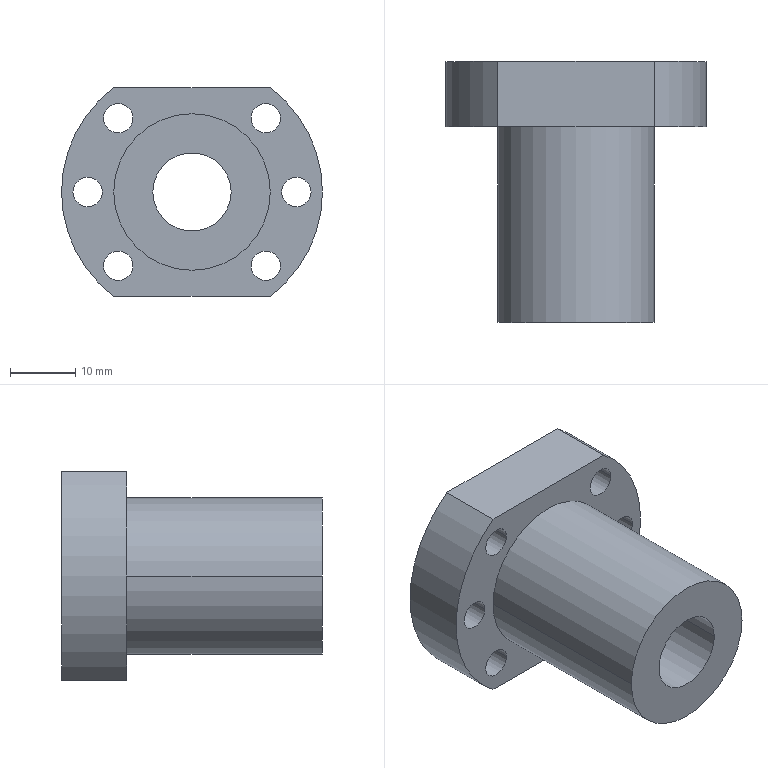Part | SolidWorks | features BaseBody 1 | 1 solid | 24 faces | box 40 x 40 x 32 mm | volume 19352 mm3 | cylinder 19 | plane 5 | commonest cylinder face diameters 4.5 x12 40 x3 12 x2 24 x2
STEP:
#1=CARTESIAN_POINT('',(-12.,-35.,0.));
#2=VERTEX_POINT('',#1);
#3=CARTESIAN_POINT('',(12.,-35.,0.));
#4=VERTEX_POINT('',#3);
#5=CARTESIAN_POINT('',(0.,-35.,0.));
#6=DIRECTION('',(0.,1.,0.));
#7=DIRECTION('',(-1.,0.,0.));
#8=AXIS2_PLACEMENT_3D('',#5,#6,#7);
#9=CIRCLE('',#8,12.);
#10=EDGE_CURVE('',#2,#4,#9,.T.);
#11=ORIENTED_EDGE('',*,*,#10,.T.);
#12=CARTESIAN_POINT('',(12.,-5.,0.));
#13=VERTEX_POINT('',#12);
#14=CARTESIAN_POINT('',(12.,-35.,0.));
#15=DIRECTION('',(0.,1.,0.));
#16=VECTOR('',#15,1000.);
#17=LINE('',#14,#16);
#18=EDGE_CURVE('',#4,#13,#17,.T.);
#19=ORIENTED_EDGE('',*,*,#18,.T.);
#20=CARTESIAN_POINT('',(-12.,-5.,0.));
#21=VERTEX_POINT('',#20);
#22=CARTESIAN_POINT('',(0.,-5.,0.));
#23=DIRECTION('',(0.,-1.,0.));
#24=DIRECTION('',(-1.,0.,0.));
#25=AXIS2_PLACEMENT_3D('',#22,#23,#24);
#26=CIRCLE('',#25,12.);
#27=EDGE_CURVE('',#13,#21,#26,.T.);
#28=ORIENTED_EDGE('',*,*,#27,.T.);
#29=CARTESIAN_POINT('',(-12.,-35.,0.));
#30=DIRECTION('',(0.,1.,0.));
#31=VECTOR('',#30,1000.);
#32=LINE('',#29,#31);
#33=EDGE_CURVE('',#2,#21,#32,.T.);
#34=ORIENTED_EDGE('',*,*,#33,.F.);
#35=EDGE_LOOP('',(#11,#19,#28,#34));
#36=FACE_OUTER_BOUND('',#35,.T.);
#37=CARTESIAN_POINT('',(0.,-35.,0.));
#38=DIRECTION('',(0.,1.,0.));
#39=DIRECTION('',(-1.,0.,0.));
#40=AXIS2_PLACEMENT_3D('',#37,#38,#39);
#41=CYLINDRICAL_SURFACE('',#40,12.);
#42=ADVANCED_FACE('',(#36),#41,.T.);
#43=CARTESIAN_POINT('',(12.,5.,-16.));
#44=VERTEX_POINT('',#43);
#45=CARTESIAN_POINT('',(20.,5.,0.));
#46=VERTEX_POINT('',#45);
#47=CARTESIAN_POINT('',(0.,5.,0.));
#48=DIRECTION('',(0.,-1.,0.));
#49=DIRECTION('',(1.,0.,0.));
#50=AXIS2_PLACEMENT_3D('',#47,#48,#49);
#51=CIRCLE('',#50,20.);
#52=EDGE_CURVE('',#44,#46,#51,.T.);
#53=ORIENTED_EDGE('',*,*,#52,.T.);
#54=CARTESIAN_POINT('',(20.,-5.,0.));
#55=VERTEX_POINT('',#54);
#56=CARTESIAN_POINT('',(20.,5.,0.));
#57=DIRECTION('',(0.,-1.,0.));
#58=VECTOR('',#57,1000.);
#59=LINE('',#56,#58);
#60=EDGE_CURVE('',#46,#55,#59,.T.);
#61=ORIENTED_EDGE('',*,*,#60,.T.);
#62=CARTESIAN_POINT('',(12.,-5.,-16.));
#63=VERTEX_POINT('',#62);
#64=CARTESIAN_POINT('',(0.,-5.,0.));
#65=DIRECTION('',(0.,1.,0.));
#66=DIRECTION('',(1.,0.,0.));
#67=AXIS2_PLACEMENT_3D('',#64,#65,#66);
#68=CIRCLE('',#67,20.);
#69=EDGE_CURVE('',#55,#63,#68,.T.);
#70=ORIENTED_EDGE('',*,*,#69,.T.);
#71=CARTESIAN_POINT('',(12.,-35.,-16.));
#72=DIRECTION('',(0.,1.,0.));
#73=VECTOR('',#72,1000.);
#74=LINE('',#71,#73);
#75=EDGE_CURVE('',#63,#44,#74,.T.);
#76=ORIENTED_EDGE('',*,*,#75,.T.);
#77=EDGE_LOOP('',(#53,#61,#70,#76));
#78=FACE_OUTER_BOUND('',#77,.T.);
#79=CARTESIAN_POINT('',(0.,5.,0.));
#80=DIRECTION('',(0.,-1.,0.));
#81=DIRECTION('',(1.,0.,0.));
#82=AXIS2_PLACEMENT_3D('',#79,#80,#81);
#83=CYLINDRICAL_SURFACE('',#82,20.);
#84=ADVANCED_FACE('',(#78),#83,.T.);
#85=CARTESIAN_POINT('',(-13.564,-5.,-11.314));
#86=VERTEX_POINT('',#85);
#87=CARTESIAN_POINT('',(-9.064,-5.,-11.314));
#88=VERTEX_POINT('',#87);
#89=CARTESIAN_POINT('',(-11.314,-5.,-11.314));
#90=DIRECTION('',(0.,-1.,0.));
#91=DIRECTION('',(-1.,0.,0.));
#92=AXIS2_PLACEMENT_3D('',#89,#90,#91);
#93=CIRCLE('',#92,2.25);
#94=EDGE_CURVE('',#86,#88,#93,.T.);
#95=ORIENTED_EDGE('',*,*,#94,.T.);
#96=CARTESIAN_POINT('',(-9.064,5.,-11.314));
#97=VERTEX_POINT('',#96);
#98=CARTESIAN_POINT('',(-9.064,-35.,-11.314));
#99=DIRECTION('',(0.,1.,0.));
#100=VECTOR('',#99,1000.);
#101=LINE('',#98,#100);
#102=EDGE_CURVE('',#88,#97,#101,.T.);
#103=ORIENTED_EDGE('',*,*,#102,.T.);
#104=CARTESIAN_POINT('',(-13.564,5.,-11.314));
#105=VERTEX_POINT('',#104);
#106=CARTESIAN_POINT('',(-11.314,5.,-11.314));
#107=DIRECTION('',(0.,-1.,0.));
#108=DIRECTION('',(-1.,0.,0.));
#109=AXIS2_PLACEMENT_3D('',#106,#107,#108);
#110=CIRCLE('',#109,2.25);
#111=EDGE_CURVE('',#105,#97,#110,.T.);
#112=ORIENTED_EDGE('',*,*,#111,.F.);
#113=CARTESIAN_POINT('',(-13.564,-35.,-11.314));
#114=DIRECTION('',(0.,1.,0.));
#115=VECTOR('',#114,1000.);
#116=LINE('',#113,#115);
#117=EDGE_CURVE('',#86,#105,#116,.T.);
#118=ORIENTED_EDGE('',*,*,#117,.F.);
#119=EDGE_LOOP('',(#95,#103,#112,#118));
#120=FACE_OUTER_BOUND('',#119,.T.);
#121=CARTESIAN_POINT('',(-11.314,-35.,-11.314));
#122=DIRECTION('',(0.,1.,0.));
#123=DIRECTION('',(-1.,0.,0.));
#124=AXIS2_PLACEMENT_3D('',#121,#122,#123);
#125=CYLINDRICAL_SURFACE('',#124,2.25);
#126=ADVANCED_FACE('',(#120),#125,.F.);
#127=CARTESIAN_POINT('',(-13.564,-5.,11.314));
#128=VERTEX_POINT('',#127);
#129=CARTESIAN_POINT('',(-9.064,-5.,11.314));
#130=VERTEX_POINT('',#129);
#131=CARTESIAN_POINT('',(-11.314,-5.,11.314));
#132=DIRECTION('',(0.,-1.,0.));
#133=DIRECTION('',(-1.,0.,0.));
#134=AXIS2_PLACEMENT_3D('',#131,#132,#133);
#135=CIRCLE('',#134,2.25);
#136=EDGE_CURVE('',#128,#130,#135,.T.);
#137=ORIENTED_EDGE('',*,*,#136,.T.);
#138=CARTESIAN_POINT('',(-9.064,5.,11.314));
#139=VERTEX_POINT('',#138);
#140=CARTESIAN_POINT('',(-9.064,-35.,11.314));
#141=DIRECTION('',(0.,1.,0.));
#142=VECTOR('',#141,1000.);
#143=LINE('',#140,#142);
#144=EDGE_CURVE('',#130,#139,#143,.T.);
#145=ORIENTED_EDGE('',*,*,#144,.T.);
#146=CARTESIAN_POINT('',(-13.564,5.,11.314));
#147=VERTEX_POINT('',#146);
#148=CARTESIAN_POINT('',(-11.314,5.,11.314));
#149=DIRECTION('',(0.,-1.,0.));
#150=DIRECTION('',(-1.,0.,0.));
#151=AXIS2_PLACEMENT_3D('',#148,#149,#150);
#152=CIRCLE('',#151,2.25);
#153=EDGE_CURVE('',#147,#139,#152,.T.);
#154=ORIENTED_EDGE('',*,*,#153,.F.);
#155=CARTESIAN_POINT('',(-13.564,-35.,11.314));
#156=DIRECTION('',(0.,1.,0.));
#157=VECTOR('',#156,1000.);
#158=LINE('',#155,#157);
#159=EDGE_CURVE('',#128,#147,#158,.T.);
#160=ORIENTED_EDGE('',*,*,#159,.F.);
#161=EDGE_LOOP('',(#137,#145,#154,#160));
#162=FACE_OUTER_BOUND('',#161,.T.);
#163=CARTESIAN_POINT('',(-11.314,-35.,11.314));
#164=DIRECTION('',(0.,1.,0.));
#165=DIRECTION('',(-1.,0.,0.));
#166=AXIS2_PLACEMENT_3D('',#163,#164,#165);
#167=CYLINDRICAL_SURFACE('',#166,2.25);
#168=ADVANCED_FACE('',(#162),#167,.F.);
#169=CARTESIAN_POINT('',(9.064,-5.,11.314));
#170=VERTEX_POINT('',#169);
#171=CARTESIAN_POINT('',(13.564,-5.,11.314));
#172=VERTEX_POINT('',#171);
#173=CARTESIAN_POINT('',(11.314,-5.,11.314));
#174=DIRECTION('',(0.,-1.,0.));
#175=DIRECTION('',(-1.,0.,0.));
#176=AXIS2_PLACEMENT_3D('',#173,#174,#175);
#177=CIRCLE('',#176,2.25);
#178=EDGE_CURVE('',#170,#172,#177,.T.);
#179=ORIENTED_EDGE('',*,*,#178,.T.);
#180=CARTESIAN_POINT('',(13.564,5.,11.314));
#181=VERTEX_POINT('',#180);
#182=CARTESIAN_POINT('',(13.564,-35.,11.314));
#183=DIRECTION('',(0.,1.,0.));
#184=VECTOR('',#183,1000.);
#185=LINE('',#182,#184);
#186=EDGE_CURVE('',#172,#181,#185,.T.);
#187=ORIENTED_EDGE('',*,*,#186,.T.);
#188=CARTESIAN_POINT('',(9.064,5.,11.314));
#189=VERTEX_POINT('',#188);
#190=CARTESIAN_POINT('',(11.314,5.,11.314));
#191=DIRECTION('',(0.,-1.,0.));
#192=DIRECTION('',(-1.,0.,0.));
#193=AXIS2_PLACEMENT_3D('',#190,#191,#192);
#194=CIRCLE('',#193,2.25);
#195=EDGE_CURVE('',#189,#181,#194,.T.);
#196=ORIENTED_EDGE('',*,*,#195,.F.);
#197=CARTESIAN_POINT('',(9.064,-35.,11.314));
#198=DIRECTION('',(0.,1.,0.));
#199=VECTOR('',#198,1000.);
#200=LINE('',#197,#199);
#201=EDGE_CURVE('',#170,#189,#200,.T.);
#202=ORIENTED_EDGE('',*,*,#201,.F.);
#203=EDGE_LOOP('',(#179,#187,#196,#202));
#204=FACE_OUTER_BOUND('',#203,.T.);
#205=CARTESIAN_POINT('',(11.314,-35.,11.314));
#206=DIRECTION('',(0.,1.,0.));
#207=DIRECTION('',(-1.,0.,0.));
#208=AXIS2_PLACEMENT_3D('',#205,#206,#207);
#209=CYLINDRICAL_SURFACE('',#208,2.25);
#210=ADVANCED_FACE('',(#204),#209,.F.);
#211=CARTESIAN_POINT('',(13.75,-5.,0.));
#212=VERTEX_POINT('',#211);
#213=CARTESIAN_POINT('',(18.25,-5.,0.));
#214=VERTEX_POINT('',#213);
#215=CARTESIAN_POINT('',(16.,-5.,0.));
#216=DIRECTION('',(0.,-1.,0.));
#217=DIRECTION('',(-1.,0.,0.));
#218=AXIS2_PLACEMENT_3D('',#215,#216,#217);
#219=CIRCLE('',#218,2.25);
#220=EDGE_CURVE('',#212,#214,#219,.T.);
#221=ORIENTED_EDGE('',*,*,#220,.T.);
#222=CARTESIAN_POINT('',(18.25,5.,0.));
#223=VERTEX_POINT('',#222);
#224=CARTESIAN_POINT('',(18.25,-35.,0.));
#225=DIRECTION('',(0.,1.,0.));
#226=VECTOR('',#225,1000.);
#227=LINE('',#224,#226);
#228=EDGE_CURVE('',#214,#223,#227,.T.);
#229=ORIENTED_EDGE('',*,*,#228,.T.);
#230=CARTESIAN_POINT('',(13.75,5.,0.));
#231=VERTEX_POINT('',#230);
#232=CARTESIAN_POINT('',(16.,5.,0.));
#233=DIRECTION('',(0.,-1.,0.));
#234=DIRECTION('',(-1.,0.,0.));
#235=AXIS2_PLACEMENT_3D('',#232,#233,#234);
#236=CIRCLE('',#235,2.25);
#237=EDGE_CURVE('',#231,#223,#236,.T.);
#238=ORIENTED_EDGE('',*,*,#237,.F.);
#239=CARTESIAN_POINT('',(13.75,-35.,0.));
#240=DIRECTION('',(0.,1.,0.));
#241=VECTOR('',#240,1000.);
#242=LINE('',#239,#241);
#243=EDGE_CURVE('',#212,#231,#242,.T.);
#244=ORIENTED_EDGE('',*,*,#243,.F.);
#245=EDGE_LOOP('',(#221,#229,#238,#244));
#246=FACE_OUTER_BOUND('',#245,.T.);
#247=CARTESIAN_POINT('',(16.,-35.,0.));
#248=DIRECTION('',(0.,1.,0.));
#249=DIRECTION('',(-1.,0.,0.));
#250=AXIS2_PLACEMENT_3D('',#247,#248,#249);
#251=CYLINDRICAL_SURFACE('',#250,2.25);
#252=ADVANCED_FACE('',(#246),#251,.F.);
#253=CARTESIAN_POINT('',(9.064,-5.,-11.314));
#254=VERTEX_POINT('',#253);
#255=CARTESIAN_POINT('',(13.564,-5.,-11.314));
#256=VERTEX_POINT('',#255);
#257=CARTESIAN_POINT('',(11.314,-5.,-11.314));
#258=DIRECTION('',(0.,-1.,0.));
#259=DIRECTION('',(-1.,0.,0.));
#260=AXIS2_PLACEMENT_3D('',#257,#258,#259);
#261=CIRCLE('',#260,2.25);
#262=EDGE_CURVE('',#254,#256,#261,.T.);
#263=ORIENTED_EDGE('',*,*,#262,.T.);
#264=CARTESIAN_POINT('',(13.564,5.,-11.314));
#265=VERTEX_POINT('',#264);
#266=CARTESIAN_POINT('',(13.564,-35.,-11.314));
#267=DIRECTION('',(0.,1.,0.));
#268=VECTOR('',#267,1000.);
#269=LINE('',#266,#268);
#270=EDGE_CURVE('',#256,#265,#269,.T.);
#271=ORIENTED_EDGE('',*,*,#270,.T.);
#272=CARTESIAN_POINT('',(9.064,5.,-11.314));
#273=VERTEX_POINT('',#272);
#274=CARTESIAN_POINT('',(11.314,5.,-11.314));
#275=DIRECTION('',(0.,-1.,0.));
#276=DIRECTION('',(-1.,0.,0.));
#277=AXIS2_PLACEMENT_3D('',#274,#275,#276);
#278=CIRCLE('',#277,2.25);
#279=EDGE_CURVE('',#273,#265,#278,.T.);
#280=ORIENTED_EDGE('',*,*,#279,.F.);
#281=CARTESIAN_POINT('',(9.064,-35.,-11.314));
#282=DIRECTION('',(0.,1.,0.));
#283=VECTOR('',#282,1000.);
#284=LINE('',#281,#283);
#285=EDGE_CURVE('',#254,#273,#284,.T.);
#286=ORIENTED_EDGE('',*,*,#285,.F.);
#287=EDGE_LOOP('',(#263,#271,#280,#286));
#288=FACE_OUTER_BOUND('',#287,.T.);
#289=CARTESIAN_POINT('',(11.314,-35.,-11.314));
#290=DIRECTION('',(0.,1.,0.));
#291=DIRECTION('',(-1.,0.,0.));
#292=AXIS2_PLACEMENT_3D('',#289,#290,#291);
#293=CYLINDRICAL_SURFACE('',#292,2.25);
#294=ADVANCED_FACE('',(#288),#293,.F.);
#295=CARTESIAN_POINT('',(-18.25,-5.,0.));
#296=VERTEX_POINT('',#295);
#297=CARTESIAN_POINT('',(-13.75,-5.,0.));
#298=VERTEX_POINT('',#297);
#299=CARTESIAN_POINT('',(-16.,-5.,0.));
#300=DIRECTION('',(0.,-1.,0.));
#301=DIRECTION('',(-1.,0.,0.));
#302=AXIS2_PLACEMENT_3D('',#299,#300,#301);
#303=CIRCLE('',#302,2.25);
#304=EDGE_CURVE('',#296,#298,#303,.T.);
#305=ORIENTED_EDGE('',*,*,#304,.T.);
#306=CARTESIAN_POINT('',(-13.75,5.,0.));
#307=VERTEX_POINT('',#306);
#308=CARTESIAN_POINT('',(-13.75,-35.,0.));
#309=DIRECTION('',(0.,1.,0.));
#310=VECTOR('',#309,1000.);
#311=LINE('',#308,#310);
#312=EDGE_CURVE('',#298,#307,#311,.T.);
#313=ORIENTED_EDGE('',*,*,#312,.T.);
#314=CARTESIAN_POINT('',(-18.25,5.,0.));
#315=VERTEX_POINT('',#314);
#316=CARTESIAN_POINT('',(-16.,5.,0.));
#317=DIRECTION('',(0.,-1.,0.));
#318=DIRECTION('',(-1.,0.,0.));
#319=AXIS2_PLACEMENT_3D('',#316,#317,#318);
#320=CIRCLE('',#319,2.25);
#321=EDGE_CURVE('',#315,#307,#320,.T.);
#322=ORIENTED_EDGE('',*,*,#321,.F.);
#323=CARTESIAN_POINT('',(-18.25,-35.,0.));
#324=DIRECTION('',(0.,1.,0.));
#325=VECTOR('',#324,1000.);
#326=LINE('',#323,#325);
#327=EDGE_CURVE('',#296,#315,#326,.T.);
#328=ORIENTED_EDGE('',*,*,#327,.F.);
#329=EDGE_LOOP('',(#305,#313,#322,#328));
#330=FACE_OUTER_BOUND('',#329,.T.);
#331=CARTESIAN_POINT('',(-16.,-35.,0.));
#332=DIRECTION('',(0.,1.,0.));
#333=DIRECTION('',(-1.,0.,0.));
#334=AXIS2_PLACEMENT_3D('',#331,#332,#333);
#335=CYLINDRICAL_SURFACE('',#334,2.25);
#336=ADVANCED_FACE('',(#330),#335,.F.);
#337=CARTESIAN_POINT('',(-6.,5.,0.));
#338=VERTEX_POINT('',#337);
#339=CARTESIAN_POINT('',(6.,5.,0.));
#340=VERTEX_POINT('',#339);
#341=CARTESIAN_POINT('',(0.,5.,0.));
#342=DIRECTION('',(0.,-1.,0.));
#343=DIRECTION('',(1.,0.,0.));
#344=AXIS2_PLACEMENT_3D('',#341,#342,#343);
#345=CIRCLE('',#344,6.);
#346=EDGE_CURVE('',#338,#340,#345,.T.);
#347=ORIENTED_EDGE('',*,*,#346,.F.);
#348=CARTESIAN_POINT('',(-6.,-35.,0.));
#349=VERTEX_POINT('',#348);
#350=CARTESIAN_POINT('',(-6.,5.,0.));
#351=DIRECTION('',(0.,-1.,0.));
#352=VECTOR('',#351,1000.);
#353=LINE('',#350,#352);
#354=EDGE_CURVE('',#338,#349,#353,.T.);
#355=ORIENTED_EDGE('',*,*,#354,.T.);
#356=CARTESIAN_POINT('',(6.,-35.,0.));
#357=VERTEX_POINT('',#356);
#358=CARTESIAN_POINT('',(0.,-35.,0.));
#359=DIRECTION('',(0.,1.,0.));
#360=DIRECTION('',(1.,0.,0.));
#361=AXIS2_PLACEMENT_3D('',#358,#359,#360);
#362=CIRCLE('',#361,6.);
#363=EDGE_CURVE('',#357,#349,#362,.T.);
#364=ORIENTED_EDGE('',*,*,#363,.F.);
#365=CARTESIAN_POINT('',(6.,5.,0.));
#366=DIRECTION('',(0.,-1.,0.));
#367=VECTOR('',#366,1000.);
#368=LINE('',#365,#367);
#369=EDGE_CURVE('',#340,#357,#368,.T.);
#370=ORIENTED_EDGE('',*,*,#369,.F.);
#371=EDGE_LOOP('',(#347,#355,#364,#370));
#372=FACE_OUTER_BOUND('',#371,.T.);
#373=CARTESIAN_POINT('',(0.,5.,0.));
#374=DIRECTION('',(0.,-1.,0.));
#375=DIRECTION('',(1.,0.,0.));
#376=AXIS2_PLACEMENT_3D('',#373,#374,#375);
#377=CYLINDRICAL_SURFACE('',#376,6.);
#378=ADVANCED_FACE('',(#372),#377,.F.);
#379=ORIENTED_EDGE('',*,*,#18,.F.);
#380=CARTESIAN_POINT('',(0.,-35.,0.));
#381=DIRECTION('',(0.,1.,0.));
#382=DIRECTION('',(-1.,0.,0.));
#383=AXIS2_PLACEMENT_3D('',#380,#381,#382);
#384=CIRCLE('',#383,12.);
#385=EDGE_CURVE('',#4,#2,#384,.T.);
#386=ORIENTED_EDGE('',*,*,#385,.T.);
#387=ORIENTED_EDGE('',*,*,#33,.T.);
#388=CARTESIAN_POINT('',(0.,-5.,0.));
#389=DIRECTION('',(0.,-1.,0.));
#390=DIRECTION('',(-1.,0.,0.));
#391=AXIS2_PLACEMENT_3D('',#388,#389,#390);
#392=CIRCLE('',#391,12.);
#393=EDGE_CURVE('',#21,#13,#392,.T.);
#394=ORIENTED_EDGE('',*,*,#393,.T.);
#395=EDGE_LOOP('',(#379,#386,#387,#394));
#396=FACE_OUTER_BOUND('',#395,.T.);
#397=CARTESIAN_POINT('',(0.,-35.,0.));
#398=DIRECTION('',(0.,1.,0.));
#399=DIRECTION('',(-1.,0.,0.));
#400=AXIS2_PLACEMENT_3D('',#397,#398,#399);
#401=CYLINDRICAL_SURFACE('',#400,12.);
#402=ADVANCED_FACE('',(#396),#401,.T.);
#403=CARTESIAN_POINT('',(-12.,-5.,-16.));
#404=VERTEX_POINT('',#403);
#405=CARTESIAN_POINT('',(0.,-5.,-16.));
#406=DIRECTION('',(-1.,0.,0.));
#407=VECTOR('',#406,1000.);
#408=LINE('',#405,#407);
#409=EDGE_CURVE('',#63,#404,#408,.T.);
#410=ORIENTED_EDGE('',*,*,#409,.F.);
#411=ORIENTED_EDGE('',*,*,#69,.F.);
#412=CARTESIAN_POINT('',(12.,-5.,16.));
#413=VERTEX_POINT('',#412);
#414=CARTESIAN_POINT('',(0.,-5.,0.));
#415=DIRECTION('',(0.,1.,0.));
#416=DIRECTION('',(1.,0.,0.));
#417=AXIS2_PLACEMENT_3D('',#414,#415,#416);
#418=CIRCLE('',#417,20.);
#419=EDGE_CURVE('',#413,#55,#418,.T.);
#420=ORIENTED_EDGE('',*,*,#419,.F.);
#421=CARTESIAN_POINT('',(-12.,-5.,16.));
#422=VERTEX_POINT('',#421);
#423=CARTESIAN_POINT('',(0.,-5.,16.));
#424=DIRECTION('',(1.,0.,0.));
#425=VECTOR('',#424,1000.);
#426=LINE('',#423,#425);
#427=EDGE_CURVE('',#422,#413,#426,.T.);
#428=ORIENTED_EDGE('',*,*,#427,.F.);
#429=CARTESIAN_POINT('',(0.,-5.,0.));
#430=DIRECTION('',(0.,1.,0.));
#431=DIRECTION('',(1.,0.,0.));
#432=AXIS2_PLACEMENT_3D('',#429,#430,#431);
#433=CIRCLE('',#432,20.);
#434=EDGE_CURVE('',#404,#422,#433,.T.);
#435=ORIENTED_EDGE('',*,*,#434,.F.);
#436=EDGE_LOOP('',(#410,#411,#420,#428,#435));
#437=FACE_OUTER_BOUND('',#436,.T.);
#438=ORIENTED_EDGE('',*,*,#393,.F.);
#439=ORIENTED_EDGE('',*,*,#27,.F.);
#440=EDGE_LOOP('',(#438,#439));
#441=FACE_BOUND('',#440,.T.);
#442=ORIENTED_EDGE('',*,*,#94,.F.);
#443=CARTESIAN_POINT('',(-11.314,-5.,-11.314));
#444=DIRECTION('',(0.,-1.,0.));
#445=DIRECTION('',(-1.,0.,0.));
#446=AXIS2_PLACEMENT_3D('',#443,#444,#445);
#447=CIRCLE('',#446,2.25);
#448=EDGE_CURVE('',#88,#86,#447,.T.);
#449=ORIENTED_EDGE('',*,*,#448,.F.);
#450=EDGE_LOOP('',(#442,#449));
#451=FACE_BOUND('',#450,.T.);
#452=ORIENTED_EDGE('',*,*,#136,.F.);
#453=CARTESIAN_POINT('',(-11.314,-5.,11.314));
#454=DIRECTION('',(0.,-1.,0.));
#455=DIRECTION('',(-1.,0.,0.));
#456=AXIS2_PLACEMENT_3D('',#453,#454,#455);
#457=CIRCLE('',#456,2.25);
#458=EDGE_CURVE('',#130,#128,#457,.T.);
#459=ORIENTED_EDGE('',*,*,#458,.F.);
#460=EDGE_LOOP('',(#452,#459));
#461=FACE_BOUND('',#460,.T.);
#462=ORIENTED_EDGE('',*,*,#178,.F.);
#463=CARTESIAN_POINT('',(11.314,-5.,11.314));
#464=DIRECTION('',(0.,-1.,0.));
#465=DIRECTION('',(-1.,0.,0.));
#466=AXIS2_PLACEMENT_3D('',#463,#464,#465);
#467=CIRCLE('',#466,2.25);
#468=EDGE_CURVE('',#172,#170,#467,.T.);
#469=ORIENTED_EDGE('',*,*,#468,.F.);
#470=EDGE_LOOP('',(#462,#469));
#471=FACE_BOUND('',#470,.T.);
#472=ORIENTED_EDGE('',*,*,#220,.F.);
#473=CARTESIAN_POINT('',(16.,-5.,0.));
#474=DIRECTION('',(0.,-1.,0.));
#475=DIRECTION('',(-1.,0.,0.));
#476=AXIS2_PLACEMENT_3D('',#473,#474,#475);
#477=CIRCLE('',#476,2.25);
#478=EDGE_CURVE('',#214,#212,#477,.T.);
#479=ORIENTED_EDGE('',*,*,#478,.F.);
#480=EDGE_LOOP('',(#472,#479));
#481=FACE_BOUND('',#480,.T.);
#482=ORIENTED_EDGE('',*,*,#262,.F.);
#483=CARTESIAN_POINT('',(11.314,-5.,-11.314));
#484=DIRECTION('',(0.,-1.,0.));
#485=DIRECTION('',(-1.,0.,0.));
#486=AXIS2_PLACEMENT_3D('',#483,#484,#485);
#487=CIRCLE('',#486,2.25);
#488=EDGE_CURVE('',#256,#254,#487,.T.);
#489=ORIENTED_EDGE('',*,*,#488,.F.);
#490=EDGE_LOOP('',(#482,#489));
#491=FACE_BOUND('',#490,.T.);
#492=ORIENTED_EDGE('',*,*,#304,.F.);
#493=CARTESIAN_POINT('',(-16.,-5.,0.));
#494=DIRECTION('',(0.,-1.,0.));
#495=DIRECTION('',(-1.,0.,0.));
#496=AXIS2_PLACEMENT_3D('',#493,#494,#495);
#497=CIRCLE('',#496,2.25);
#498=EDGE_CURVE('',#298,#296,#497,.T.);
#499=ORIENTED_EDGE('',*,*,#498,.F.);
#500=EDGE_LOOP('',(#492,#499));
#501=FACE_BOUND('',#500,.T.);
#502=CARTESIAN_POINT('',(0.,-5.,0.));
#503=DIRECTION('',(0.,1.,0.));
#504=DIRECTION('',(-1.,0.,0.));
#505=AXIS2_PLACEMENT_3D('',#502,#503,#504);
#506=PLANE('',#505);
#507=ADVANCED_FACE('',(#437,#441,#451,#461,#471,#481,#491,#501),#506,.F.);
#508=ORIENTED_EDGE('',*,*,#10,.F.);
#509=ORIENTED_EDGE('',*,*,#385,.F.);
#510=EDGE_LOOP('',(#508,#509));
#511=FACE_OUTER_BOUND('',#510,.T.);
#512=ORIENTED_EDGE('',*,*,#363,.T.);
#513=CARTESIAN_POINT('',(0.,-35.,0.));
#514=DIRECTION('',(0.,1.,0.));
#515=DIRECTION('',(1.,0.,0.));
#516=AXIS2_PLACEMENT_3D('',#513,#514,#515);
#517=CIRCLE('',#516,6.);
#518=EDGE_CURVE('',#349,#357,#517,.T.);
#519=ORIENTED_EDGE('',*,*,#518,.T.);
#520=EDGE_LOOP('',(#512,#519));
#521=FACE_BOUND('',#520,.T.);
#522=CARTESIAN_POINT('',(0.,-35.,0.));
#523=DIRECTION('',(0.,-1.,0.));
#524=DIRECTION('',(1.,0.,0.));
#525=AXIS2_PLACEMENT_3D('',#522,#523,#524);
#526=PLANE('',#525);
#527=ADVANCED_FACE('',(#511,#521),#526,.T.);
#528=ORIENTED_EDGE('',*,*,#434,.T.);
#529=CARTESIAN_POINT('',(-12.,5.,16.));
#530=VERTEX_POINT('',#529);
#531=CARTESIAN_POINT('',(-12.,5.,16.));
#532=DIRECTION('',(0.,1.,0.));
#533=VECTOR('',#532,1000.);
#534=LINE('',#531,#533);
#535=EDGE_CURVE('',#422,#530,#534,.T.);
#536=ORIENTED_EDGE('',*,*,#535,.T.);
#537=CARTESIAN_POINT('',(-12.,5.,-16.));
#538=VERTEX_POINT('',#537);
#539=CARTESIAN_POINT('',(0.,5.,0.));
#540=DIRECTION('',(0.,-1.,0.));
#541=DIRECTION('',(1.,0.,0.));
#542=AXIS2_PLACEMENT_3D('',#539,#540,#541);
#543=CIRCLE('',#542,20.);
#544=EDGE_CURVE('',#530,#538,#543,.T.);
#545=ORIENTED_EDGE('',*,*,#544,.T.);
#546=CARTESIAN_POINT('',(-12.,5.,-16.));
#547=DIRECTION('',(0.,-1.,0.));
#548=VECTOR('',#547,1000.);
#549=LINE('',#546,#548);
#550=EDGE_CURVE('',#538,#404,#549,.T.);
#551=ORIENTED_EDGE('',*,*,#550,.T.);
#552=EDGE_LOOP('',(#528,#536,#545,#551));
#553=FACE_OUTER_BOUND('',#552,.T.);
#554=CARTESIAN_POINT('',(0.,5.,0.));
#555=DIRECTION('',(0.,-1.,0.));
#556=DIRECTION('',(1.,0.,0.));
#557=AXIS2_PLACEMENT_3D('',#554,#555,#556);
#558=CYLINDRICAL_SURFACE('',#557,20.);
#559=ADVANCED_FACE('',(#553),#558,.T.);
#560=CARTESIAN_POINT('',(-12.,5.,-16.));
#561=DIRECTION('',(-1.,0.,0.));
#562=VECTOR('',#561,1000.);
#563=LINE('',#560,#562);
#564=EDGE_CURVE('',#44,#538,#563,.T.);
#565=ORIENTED_EDGE('',*,*,#564,.F.);
#566=ORIENTED_EDGE('',*,*,#75,.F.);
#567=ORIENTED_EDGE('',*,*,#409,.T.);
#568=ORIENTED_EDGE('',*,*,#550,.F.);
#569=EDGE_LOOP('',(#565,#566,#567,#568));
#570=FACE_OUTER_BOUND('',#569,.T.);
#571=CARTESIAN_POINT('',(-12.,-35.,-16.));
#572=DIRECTION('',(0.,0.,1.));
#573=DIRECTION('',(1.,0.,0.));
#574=AXIS2_PLACEMENT_3D('',#571,#572,#573);
#575=PLANE('',#574);
#576=ADVANCED_FACE('',(#570),#575,.F.);
#577=ORIENTED_EDGE('',*,*,#60,.F.);
#578=CARTESIAN_POINT('',(12.,5.,16.));
#579=VERTEX_POINT('',#578);
#580=CARTESIAN_POINT('',(0.,5.,0.));
#581=DIRECTION('',(0.,-1.,0.));
#582=DIRECTION('',(1.,0.,0.));
#583=AXIS2_PLACEMENT_3D('',#580,#581,#582);
#584=CIRCLE('',#583,20.);
#585=EDGE_CURVE('',#46,#579,#584,.T.);
#586=ORIENTED_EDGE('',*,*,#585,.T.);
#587=CARTESIAN_POINT('',(12.,5.,16.));
#588=DIRECTION('',(0.,-1.,0.));
#589=VECTOR('',#588,1000.);
#590=LINE('',#587,#589);
#591=EDGE_CURVE('',#579,#413,#590,.T.);
#592=ORIENTED_EDGE('',*,*,#591,.T.);
#593=ORIENTED_EDGE('',*,*,#419,.T.);
#594=EDGE_LOOP('',(#577,#586,#592,#593));
#595=FACE_OUTER_BOUND('',#594,.T.);
#596=CARTESIAN_POINT('',(0.,5.,0.));
#597=DIRECTION('',(0.,-1.,0.));
#598=DIRECTION('',(1.,0.,0.));
#599=AXIS2_PLACEMENT_3D('',#596,#597,#598);
#600=CYLINDRICAL_SURFACE('',#599,20.);
#601=ADVANCED_FACE('',(#595),#600,.T.);
#602=CARTESIAN_POINT('',(-12.,5.,16.));
#603=DIRECTION('',(1.,0.,0.));
#604=VECTOR('',#603,1000.);
#605=LINE('',#602,#604);
#606=EDGE_CURVE('',#530,#579,#605,.T.);
#607=ORIENTED_EDGE('',*,*,#606,.F.);
#608=ORIENTED_EDGE('',*,*,#535,.F.);
#609=ORIENTED_EDGE('',*,*,#427,.T.);
#610=ORIENTED_EDGE('',*,*,#591,.F.);
#611=EDGE_LOOP('',(#607,#608,#609,#610));
#612=FACE_OUTER_BOUND('',#611,.T.);
#613=CARTESIAN_POINT('',(-12.,-35.,16.));
#614=DIRECTION('',(0.,0.,-1.));
#615=DIRECTION('',(-1.,0.,0.));
#616=AXIS2_PLACEMENT_3D('',#613,#614,#615);
#617=PLANE('',#616);
#618=ADVANCED_FACE('',(#612),#617,.F.);
#619=ORIENTED_EDGE('',*,*,#102,.F.);
#620=ORIENTED_EDGE('',*,*,#448,.T.);
#621=ORIENTED_EDGE('',*,*,#117,.T.);
#622=CARTESIAN_POINT('',(-11.314,5.,-11.314));
#623=DIRECTION('',(0.,-1.,0.));
#624=DIRECTION('',(-1.,0.,0.));
#625=AXIS2_PLACEMENT_3D('',#622,#623,#624);
#626=CIRCLE('',#625,2.25);
#627=EDGE_CURVE('',#97,#105,#626,.T.);
#628=ORIENTED_EDGE('',*,*,#627,.F.);
#629=EDGE_LOOP('',(#619,#620,#621,#628));
#630=FACE_OUTER_BOUND('',#629,.T.);
#631=CARTESIAN_POINT('',(-11.314,-35.,-11.314));
#632=DIRECTION('',(0.,1.,0.));
#633=DIRECTION('',(-1.,0.,0.));
#634=AXIS2_PLACEMENT_3D('',#631,#632,#633);
#635=CYLINDRICAL_SURFACE('',#634,2.25);
#636=ADVANCED_FACE('',(#630),#635,.F.);
#637=ORIENTED_EDGE('',*,*,#144,.F.);
#638=ORIENTED_EDGE('',*,*,#458,.T.);
#639=ORIENTED_EDGE('',*,*,#159,.T.);
#640=CARTESIAN_POINT('',(-11.314,5.,11.314));
#641=DIRECTION('',(0.,-1.,0.));
#642=DIRECTION('',(-1.,0.,0.));
#643=AXIS2_PLACEMENT_3D('',#640,#641,#642);
#644=CIRCLE('',#643,2.25);
#645=EDGE_CURVE('',#139,#147,#644,.T.);
#646=ORIENTED_EDGE('',*,*,#645,.F.);
#647=EDGE_LOOP('',(#637,#638,#639,#646));
#648=FACE_OUTER_BOUND('',#647,.T.);
#649=CARTESIAN_POINT('',(-11.314,-35.,11.314));
#650=DIRECTION('',(0.,1.,0.));
#651=DIRECTION('',(-1.,0.,0.));
#652=AXIS2_PLACEMENT_3D('',#649,#650,#651);
#653=CYLINDRICAL_SURFACE('',#652,2.25);
#654=ADVANCED_FACE('',(#648),#653,.F.);
#655=ORIENTED_EDGE('',*,*,#186,.F.);
#656=ORIENTED_EDGE('',*,*,#468,.T.);
#657=ORIENTED_EDGE('',*,*,#201,.T.);
#658=CARTESIAN_POINT('',(11.314,5.,11.314));
#659=DIRECTION('',(0.,-1.,0.));
#660=DIRECTION('',(-1.,0.,0.));
#661=AXIS2_PLACEMENT_3D('',#658,#659,#660);
#662=CIRCLE('',#661,2.25);
#663=EDGE_CURVE('',#181,#189,#662,.T.);
#664=ORIENTED_EDGE('',*,*,#663,.F.);
#665=EDGE_LOOP('',(#655,#656,#657,#664));
#666=FACE_OUTER_BOUND('',#665,.T.);
#667=CARTESIAN_POINT('',(11.314,-35.,11.314));
#668=DIRECTION('',(0.,1.,0.));
#669=DIRECTION('',(-1.,0.,0.));
#670=AXIS2_PLACEMENT_3D('',#667,#668,#669);
#671=CYLINDRICAL_SURFACE('',#670,2.25);
#672=ADVANCED_FACE('',(#666),#671,.F.);
#673=ORIENTED_EDGE('',*,*,#228,.F.);
#674=ORIENTED_EDGE('',*,*,#478,.T.);
#675=ORIENTED_EDGE('',*,*,#243,.T.);
#676=CARTESIAN_POINT('',(16.,5.,0.));
#677=DIRECTION('',(0.,-1.,0.));
#678=DIRECTION('',(-1.,0.,0.));
#679=AXIS2_PLACEMENT_3D('',#676,#677,#678);
#680=CIRCLE('',#679,2.25);
#681=EDGE_CURVE('',#223,#231,#680,.T.);
#682=ORIENTED_EDGE('',*,*,#681,.F.);
#683=EDGE_LOOP('',(#673,#674,#675,#682));
#684=FACE_OUTER_BOUND('',#683,.T.);
#685=CARTESIAN_POINT('',(16.,-35.,0.));
#686=DIRECTION('',(0.,1.,0.));
#687=DIRECTION('',(-1.,0.,0.));
#688=AXIS2_PLACEMENT_3D('',#685,#686,#687);
#689=CYLINDRICAL_SURFACE('',#688,2.25);
#690=ADVANCED_FACE('',(#684),#689,.F.);
#691=ORIENTED_EDGE('',*,*,#270,.F.);
#692=ORIENTED_EDGE('',*,*,#488,.T.);
#693=ORIENTED_EDGE('',*,*,#285,.T.);
#694=CARTESIAN_POINT('',(11.314,5.,-11.314));
#695=DIRECTION('',(0.,-1.,0.));
#696=DIRECTION('',(-1.,0.,0.));
#697=AXIS2_PLACEMENT_3D('',#694,#695,#696);
#698=CIRCLE('',#697,2.25);
#699=EDGE_CURVE('',#265,#273,#698,.T.);
#700=ORIENTED_EDGE('',*,*,#699,.F.);
#701=EDGE_LOOP('',(#691,#692,#693,#700));
#702=FACE_OUTER_BOUND('',#701,.T.);
#703=CARTESIAN_POINT('',(11.314,-35.,-11.314));
#704=DIRECTION('',(0.,1.,0.));
#705=DIRECTION('',(-1.,0.,0.));
#706=AXIS2_PLACEMENT_3D('',#703,#704,#705);
#707=CYLINDRICAL_SURFACE('',#706,2.25);
#708=ADVANCED_FACE('',(#702),#707,.F.);
#709=ORIENTED_EDGE('',*,*,#312,.F.);
#710=ORIENTED_EDGE('',*,*,#498,.T.);
#711=ORIENTED_EDGE('',*,*,#327,.T.);
#712=CARTESIAN_POINT('',(-16.,5.,0.));
#713=DIRECTION('',(0.,-1.,0.));
#714=DIRECTION('',(-1.,0.,0.));
#715=AXIS2_PLACEMENT_3D('',#712,#713,#714);
#716=CIRCLE('',#715,2.25);
#717=EDGE_CURVE('',#307,#315,#716,.T.);
#718=ORIENTED_EDGE('',*,*,#717,.F.);
#719=EDGE_LOOP('',(#709,#710,#711,#718));
#720=FACE_OUTER_BOUND('',#719,.T.);
#721=CARTESIAN_POINT('',(-16.,-35.,0.));
#722=DIRECTION('',(0.,1.,0.));
#723=DIRECTION('',(-1.,0.,0.));
#724=AXIS2_PLACEMENT_3D('',#721,#722,#723);
#725=CYLINDRICAL_SURFACE('',#724,2.25);
#726=ADVANCED_FACE('',(#720),#725,.F.);
#727=ORIENTED_EDGE('',*,*,#354,.F.);
#728=CARTESIAN_POINT('',(0.,5.,0.));
#729=DIRECTION('',(0.,-1.,0.));
#730=DIRECTION('',(1.,0.,0.));
#731=AXIS2_PLACEMENT_3D('',#728,#729,#730);
#732=CIRCLE('',#731,6.);
#733=EDGE_CURVE('',#340,#338,#732,.T.);
#734=ORIENTED_EDGE('',*,*,#733,.F.);
#735=ORIENTED_EDGE('',*,*,#369,.T.);
#736=ORIENTED_EDGE('',*,*,#518,.F.);
#737=EDGE_LOOP('',(#727,#734,#735,#736));
#738=FACE_OUTER_BOUND('',#737,.T.);
#739=CARTESIAN_POINT('',(0.,5.,0.));
#740=DIRECTION('',(0.,-1.,0.));
#741=DIRECTION('',(1.,0.,0.));
#742=AXIS2_PLACEMENT_3D('',#739,#740,#741);
#743=CYLINDRICAL_SURFACE('',#742,6.);
#744=ADVANCED_FACE('',(#738),#743,.F.);
#745=ORIENTED_EDGE('',*,*,#733,.T.);
#746=ORIENTED_EDGE('',*,*,#346,.T.);
#747=EDGE_LOOP('',(#745,#746));
#748=FACE_BOUND('',#747,.T.);
#749=ORIENTED_EDGE('',*,*,#606,.T.);
#750=ORIENTED_EDGE('',*,*,#585,.F.);
#751=ORIENTED_EDGE('',*,*,#52,.F.);
#752=ORIENTED_EDGE('',*,*,#564,.T.);
#753=ORIENTED_EDGE('',*,*,#544,.F.);
#754=EDGE_LOOP('',(#749,#750,#751,#752,#753));
#755=FACE_OUTER_BOUND('',#754,.T.);
#756=ORIENTED_EDGE('',*,*,#111,.T.);
#757=ORIENTED_EDGE('',*,*,#627,.T.);
#758=EDGE_LOOP('',(#756,#757));
#759=FACE_BOUND('',#758,.T.);
#760=ORIENTED_EDGE('',*,*,#153,.T.);
#761=ORIENTED_EDGE('',*,*,#645,.T.);
#762=EDGE_LOOP('',(#760,#761));
#763=FACE_BOUND('',#762,.T.);
#764=ORIENTED_EDGE('',*,*,#195,.T.);
#765=ORIENTED_EDGE('',*,*,#663,.T.);
#766=EDGE_LOOP('',(#764,#765));
#767=FACE_BOUND('',#766,.T.);
#768=ORIENTED_EDGE('',*,*,#237,.T.);
#769=ORIENTED_EDGE('',*,*,#681,.T.);
#770=EDGE_LOOP('',(#768,#769));
#771=FACE_BOUND('',#770,.T.);
#772=ORIENTED_EDGE('',*,*,#279,.T.);
#773=ORIENTED_EDGE('',*,*,#699,.T.);
#774=EDGE_LOOP('',(#772,#773));
#775=FACE_BOUND('',#774,.T.);
#776=ORIENTED_EDGE('',*,*,#321,.T.);
#777=ORIENTED_EDGE('',*,*,#717,.T.);
#778=EDGE_LOOP('',(#776,#777));
#779=FACE_BOUND('',#778,.T.);
#780=CARTESIAN_POINT('',(0.,5.,0.));
#781=DIRECTION('',(0.,1.,0.));
#782=DIRECTION('',(-1.,0.,0.));
#783=AXIS2_PLACEMENT_3D('',#780,#781,#782);
#784=PLANE('',#783);
#785=ADVANCED_FACE('',(#748,#755,#759,#763,#767,#771,#775,#779),#784,.T.);
#786=CLOSED_SHELL('',(#42,#84,#126,#168,#210,#252,#294,#336,#378,#402,#507,#527,#559,#576,#601,#618,#636,#654,#672,#690,#708,#726,#744,#785));
#787=MANIFOLD_SOLID_BREP('',#786);
#788=CARTESIAN_POINT('',(0.,0.,0.));
#789=DIRECTION('',(0.,0.,1.));
#790=DIRECTION('',(1.,0.,0.));
#791=AXIS2_PLACEMENT_3D('',#788,#789,#790);
#792=(LENGTH_UNIT()NAMED_UNIT(*)SI_UNIT(.MILLI.,.METRE.));
#793=UNCERTAINTY_MEASURE_WITH_UNIT(LENGTH_MEASURE(0.00001),#792,'','');
#794=(NAMED_UNIT(*)PLANE_ANGLE_UNIT()SI_UNIT($,.RADIAN.));
#795=(NAMED_UNIT(*)SI_UNIT($,.STERADIAN.)SOLID_ANGLE_UNIT());
#796=(GEOMETRIC_REPRESENTATION_CONTEXT(3)GLOBAL_UNCERTAINTY_ASSIGNED_CONTEXT((#793))GLOBAL_UNIT_ASSIGNED_CONTEXT((#792,#794,#795))REPRESENTATION_CONTEXT('',''));
#797=ADVANCED_BREP_SHAPE_REPRESENTATION('',(#787,#791),#796);